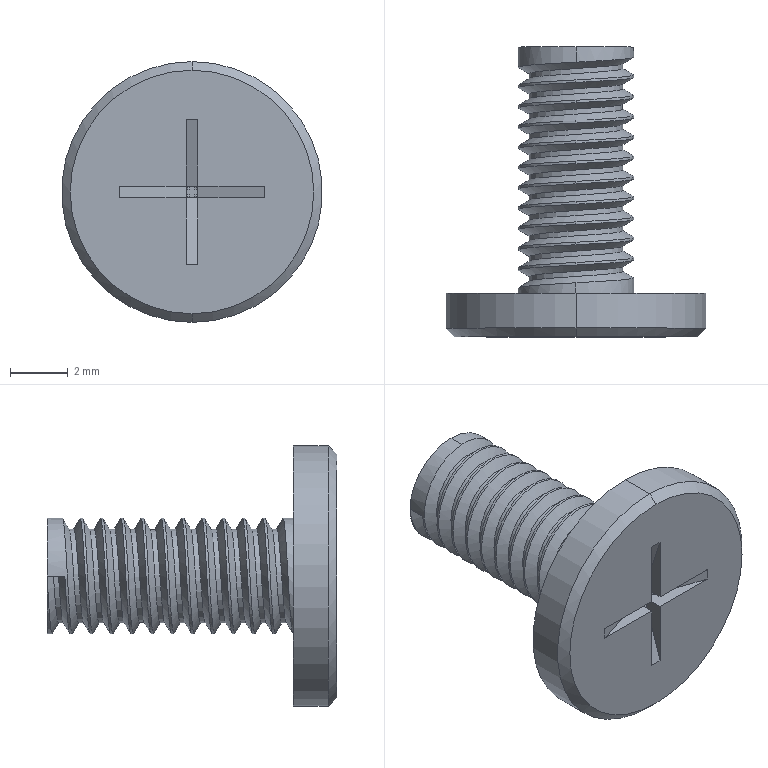Part | SolidWorks | features BaseBody 1 | 1 solid | 64 faces | box 9 x 10 x 9 mm | volume 179.425 mm3 | plane 30 | cylinder 28 | spline 4 | cone 2 | commonest cylinder face diameters 4 x26 9 x2